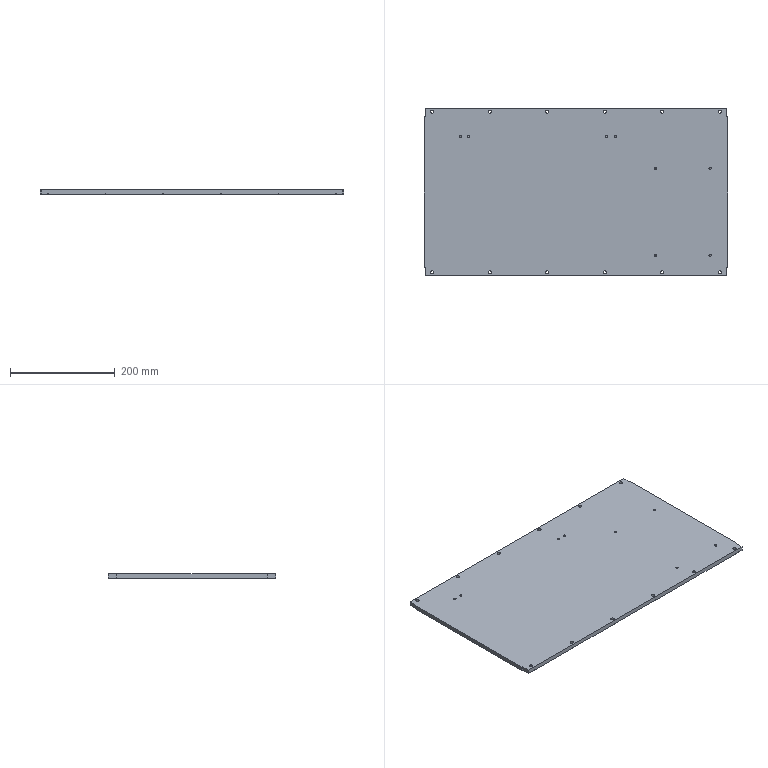Part | SolidWorks | features BaseBody 1 | 1 solid | 94 faces | box 580.05 x 320 x 8 mm | volume 1478384 mm3 | cylinder 40 | cone 40 | plane 14 | commonest cylinder face diameters 6.2 x24 4.2 x16